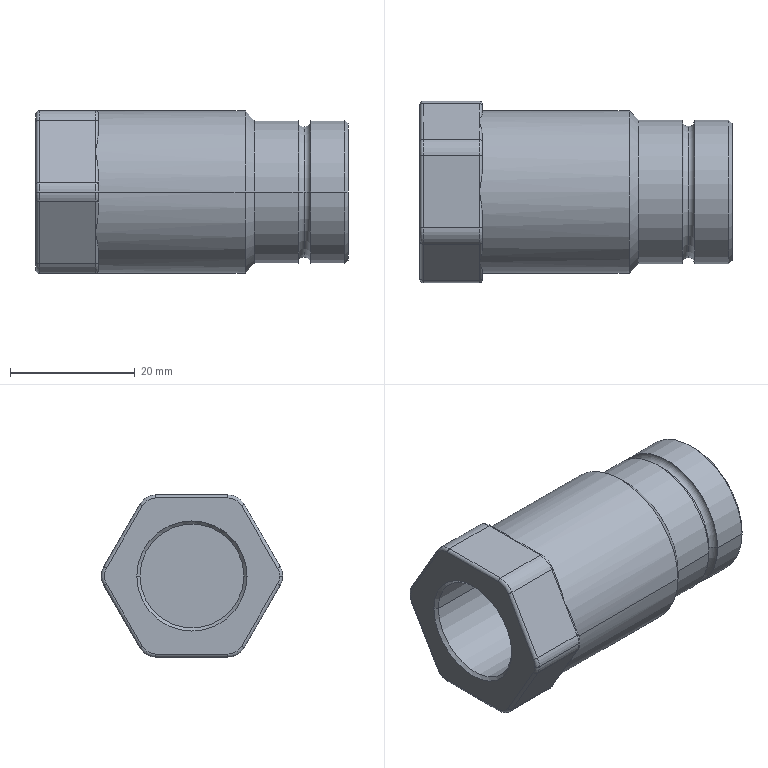Part | STEP file | 4-20.sldasm-Part-118 | 1 solid | 209 faces | box 50 x 29.094 x 26 mm | volume 17659 mm3 | plane 87 | spline 57 | cylinder 37 | torus 18 | cone 10 | commonest cylinder face diameters 1 x18 6 x7 23 x4 15 x2 16 x2 16.66 x2